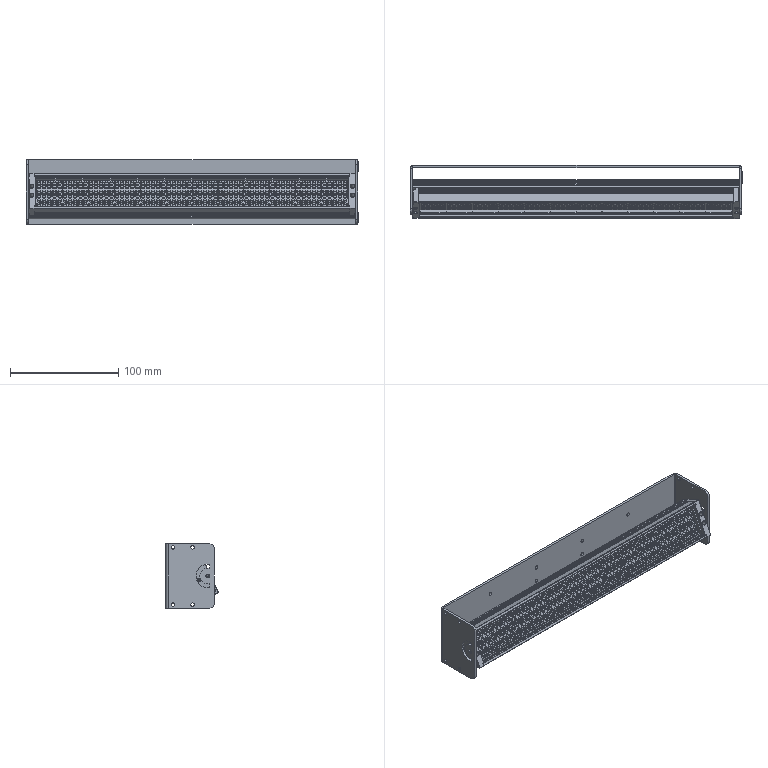Part | 16 solids | 2133 faces | box 307 x 48.966 x 60 mm | volume 133132 mm3 | spline 720 | plane 623 | cylinder 610 | cone 180 | commonest cylinder face diameters 2 x290 1.9 x144 0.2 x66 3.3 x36 0.6 x24 1.6 x10